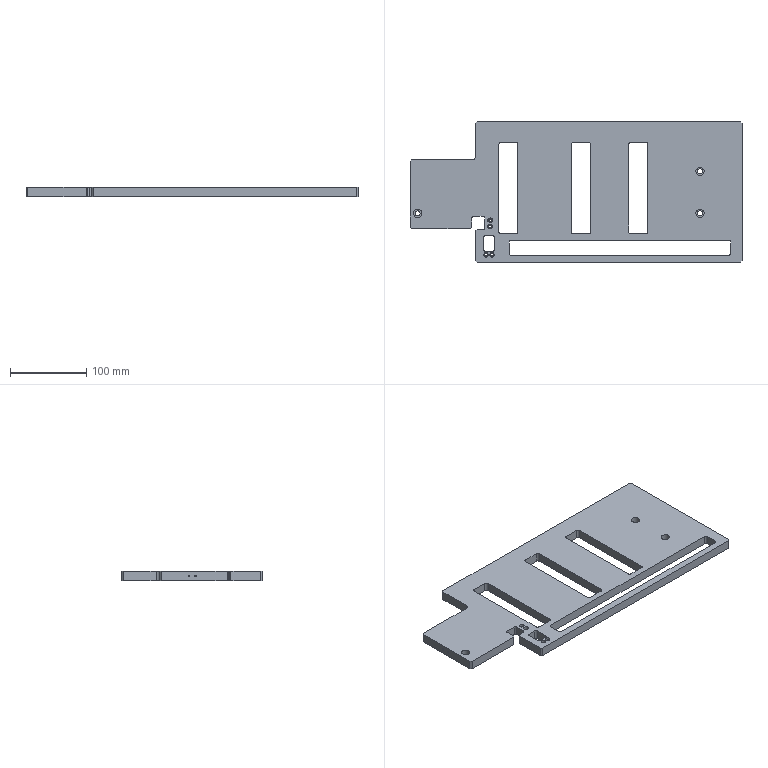NC program | NX | posted with a generic post | part box 435 x 184 x 12 mm
Lines 1 to 1792 of 10210:
N10 G17 G21 G94 G90
(DRILLING_COPY_1 , TOOL : D6A45)
N12 T01 M6
N14 G54
N16 G17 G0 G90 X-207.5 Y-28. S5000 M3
N18 G43 Z30. H1
N20 G94 G81 G98 Z-1. F350. R3.
N22 X-112.5 Y-37.
N24 Y-45.
N26 X-118. Y-82.5
N28 X-110.
N30 X162.5 Y-28.
N32 Y27.
N34 G80
N36 G0 X162.5 Y27. Z30.
N38 M5
(DRILLING_COPY_1_COPY_COPY_1 , TOOL : 3.5ZT)
N40 T07 M6
N42 G54
N44 G17 G0 G90 X-112.5 Y-37. S2000 M3
N46 G43 Z30. H7
N48 G94 G83 G98 Z-14.052 F200. Q2. R3.
N50 Y-45.
N52 X-110. Y-82.5
N54 X-118.
N56 G80
N58 G0 X-118. Y-82.5 Z30.
N60 M5
(DRILLING_COPY_1_COPY_COPY_1_COPY , TOOL : 6.5ZT)
N62 T16 M6
N64 G54
N66 G17 G0 G90 X-207.5 Y-28. S2000 M3
N68 G43 Z30. H16
N70 G94 G83 G98 Z-14.953 F200. Q2. R3.
N72 X162.5
N74 Y27.
N76 G80
N78 G0 X162.5 Y27. Z30.
N80 M5
(ZLEVEL_PROFILE_COPY_1_COPY_COPY_1_COPY , TOOL : D10)
N82 T15 M6
N84 G54
N86 G17 G0 G90 X-132.526 Y98.746 S9500 M3
N88 G43 Z30. H15
N90 Z0.
N92 G94 G1 Z-1. F1000.
N94 X-132.136 Y97.282
N96 G2 X-132.396 Y96.317 R1.
N98 G3 X-132.523 Y96.108 R0.16 F2000.
N100 X-133.106 Y95.606 R5.1
N102 G1 X-135.106 Y93.606
N104 G3 X-136.6 Y90. R5.1
N106 G1 Y47.203
N108 X-136.611 Y47.1
N110 X-215.5
N112 G3 X-219.106 Y45.606 R5.1
N114 G1 X-220.39 Y44.318
N116 X-220.664 Y44.045
N118 X-220.688 Y43.981
N120 G3 X-222.6 Y40. R5.1
N122 G1 Y-44.953
N124 X-222.597 Y-45.002
N126 Y-45.389
N128 X-222.569 Y-45.44
N130 G3 X-221.106 Y-49.606 R5.1
N132 G1 X-219.106 Y-51.606
N134 G3 X-215.5 Y-53.1 R5.1
N136 G1 X-138.5
N138 G3 X-136.6 Y-52.733 R5.1
N140 G1 Y-90.
N142 G3 X-135.106 Y-93.606 R5.1
N144 G1 X-133.106 Y-95.606
N146 G3 X-132.695 Y-95.975 R5.1
N148 G2 X-132.514 Y-96.441 R0.5
N150 G1 X-132.838 Y-98.537
N152 Z0.
N154 G0 Z54.
N156 X-132.526 Y98.746
N158 Z-1.
N160 G1 Z-2. F1000.
N162 X-132.136 Y97.282
N164 G2 X-132.396 Y96.317 R1.
N166 G3 X-132.523 Y96.108 R0.16 F2000.
N168 X-133.106 Y95.606 R5.1
N170 G1 X-135.106 Y93.606
N172 G3 X-136.6 Y90. R5.1
N174 G1 Y47.203
N176 X-136.611 Y47.1
N178 X-215.5
N180 G3 X-219.106 Y45.606 R5.1
N182 G1 X-220.39 Y44.318
N184 X-220.664 Y44.045
N186 X-220.688 Y43.981
N188 G3 X-222.6 Y40. R5.1
N190 G1 Y-44.953
N192 X-222.597 Y-45.002
N194 Y-45.389
N196 X-222.569 Y-45.44
N198 G3 X-221.106 Y-49.606 R5.1
N200 G1 X-219.106 Y-51.606
N202 G3 X-215.5 Y-53.1 R5.1
N204 G1 X-138.5
N206 G3 X-136.6 Y-52.733 R5.1
N208 G1 Y-90.
N210 G3 X-135.106 Y-93.606 R5.1
N212 G1 X-133.106 Y-95.606
N214 G3 X-132.695 Y-95.975 R5.1
N216 G2 X-132.514 Y-96.441 R0.5
N218 G1 X-132.838 Y-98.537
N220 Z-1.
N222 G0 Z54.
N224 X-132.526 Y98.746
N226 Z-2.
N228 G1 Z-3. F1000.
N230 X-132.136 Y97.282
N232 G2 X-132.396 Y96.317 R1.
N234 G3 X-132.523 Y96.108 R0.16 F2000.
N236 X-133.106 Y95.606 R5.1
N238 G1 X-135.106 Y93.606
N240 G3 X-136.6 Y90. R5.1
N242 G1 Y47.203
N244 X-136.611 Y47.1
N246 X-215.5
N248 G3 X-219.106 Y45.606 R5.1
N250 G1 X-220.39 Y44.318
N252 X-220.664 Y44.045
N254 X-220.688 Y43.981
N256 G3 X-222.6 Y40. R5.1
N258 G1 Y-44.953
N260 X-222.597 Y-45.002
N262 Y-45.389
N264 X-222.569 Y-45.44
N266 G3 X-221.106 Y-49.606 R5.1
N268 G1 X-219.106 Y-51.606
N270 G3 X-215.5 Y-53.1 R5.1
N272 G1 X-138.5
N274 G3 X-136.6 Y-52.733 R5.1
N276 G1 Y-90.
N278 G3 X-135.106 Y-93.606 R5.1
N280 G1 X-133.106 Y-95.606
N282 G3 X-132.695 Y-95.975 R5.1
N284 G2 X-132.514 Y-96.441 R0.5
N286 G1 X-132.838 Y-98.537
N288 Z-2.
N290 G0 Z54.
N292 X-132.526 Y98.746
N294 Z-3.
N296 G1 Z-4. F1000.
N298 X-132.136 Y97.282
N300 G2 X-132.396 Y96.317 R1.
N302 G3 X-132.523 Y96.108 R0.16 F2000.
N304 X-133.106 Y95.606 R5.1
N306 G1 X-135.106 Y93.606
N308 G3 X-136.6 Y90. R5.1
N310 G1 Y47.203
N312 X-136.611 Y47.1
N314 X-215.5
N316 G3 X-219.106 Y45.606 R5.1
N318 G1 X-220.39 Y44.318
N320 X-220.664 Y44.045
N322 X-220.688 Y43.981
N324 G3 X-222.6 Y40. R5.1
N326 G1 Y-44.953
N328 X-222.597 Y-45.002
N330 Y-45.389
N332 X-222.569 Y-45.44
N334 G3 X-221.106 Y-49.606 R5.1
N336 G1 X-219.106 Y-51.606
N338 G3 X-215.5 Y-53.1 R5.1
N340 G1 X-138.5
N342 G3 X-136.6 Y-52.733 R5.1
N344 G1 Y-90.
N346 G3 X-135.106 Y-93.606 R5.1
N348 G1 X-133.106 Y-95.606
N350 G3 X-132.695 Y-95.975 R5.1
N352 G2 X-132.514 Y-96.441 R0.5
N354 G1 X-132.838 Y-98.537
N356 Z-3.
N358 G0 Z54.
N360 X-132.526 Y98.746
N362 Z-4.
N364 G1 Z-5. F1000.
N366 X-132.136 Y97.282
N368 G2 X-132.396 Y96.317 R1.
N370 G3 X-132.523 Y96.108 R0.16 F2000.
N372 X-133.106 Y95.606 R5.1
N374 G1 X-135.106 Y93.606
N376 G3 X-136.6 Y90. R5.1
N378 G1 Y47.203
N380 X-136.611 Y47.1
N382 X-215.5
N384 G3 X-219.106 Y45.606 R5.1
N386 G1 X-220.39 Y44.318
N388 X-220.664 Y44.045
N390 X-220.688 Y43.981
N392 G3 X-222.6 Y40. R5.1
N394 G1 Y-44.953
N396 X-222.597 Y-45.002
N398 Y-45.389
N400 X-222.569 Y-45.44
N402 G3 X-221.106 Y-49.606 R5.1
N404 G1 X-219.106 Y-51.606
N406 G3 X-215.5 Y-53.1 R5.1
N408 G1 X-138.5
N410 G3 X-136.6 Y-52.733 R5.1
N412 G1 Y-90.
N414 G3 X-135.106 Y-93.606 R5.1
N416 G1 X-133.106 Y-95.606
N418 G3 X-132.695 Y-95.975 R5.1
N420 G2 X-132.514 Y-96.441 R0.5
N422 G1 X-132.838 Y-98.537
N424 Z-4.
N426 G0 Z54.
N428 X-132.526 Y98.746
N430 Z-5.
N432 G1 Z-6. F1000.
N434 X-132.136 Y97.282
N436 G2 X-132.396 Y96.317 R1.
N438 G3 X-132.523 Y96.108 R0.16 F2000.
N440 X-133.106 Y95.606 R5.1
N442 G1 X-135.106 Y93.606
N444 G3 X-136.6 Y90. R5.1
N446 G1 Y47.203
N448 X-136.611 Y47.1
N450 X-215.5
N452 G3 X-219.106 Y45.606 R5.1
N454 G1 X-220.39 Y44.318
N456 X-220.664 Y44.045
N458 X-220.688 Y43.981
N460 G3 X-222.6 Y40. R5.1
N462 G1 Y-44.953
N464 X-222.597 Y-45.002
N466 Y-45.389
N468 X-222.569 Y-45.44
N470 G3 X-221.106 Y-49.606 R5.1
N472 G1 X-219.106 Y-51.606
N474 G3 X-215.5 Y-53.1 R5.1
N476 G1 X-138.5
N478 G3 X-136.6 Y-52.733 R5.1
N480 G1 Y-90.
N482 G3 X-135.106 Y-93.606 R5.1
N484 G1 X-133.106 Y-95.606
N486 G3 X-132.695 Y-95.975 R5.1
N488 G2 X-132.514 Y-96.441 R0.5
N490 G1 X-132.838 Y-98.537
N492 Z-5.
N494 G0 Z54.
N496 X-132.526 Y98.746
N498 Z-6.
N500 G1 Z-7. F1000.
N502 X-132.136 Y97.282
N504 G2 X-132.396 Y96.317 R1.
N506 G3 X-132.523 Y96.108 R0.16 F2000.
N508 X-133.106 Y95.606 R5.1
N510 G1 X-135.106 Y93.606
N512 G3 X-136.6 Y90. R5.1
N514 G1 Y47.203
N516 X-136.611 Y47.1
N518 X-215.5
N520 G3 X-219.106 Y45.606 R5.1
N522 G1 X-220.39 Y44.318
N524 X-220.664 Y44.045
N526 X-220.688 Y43.981
N528 G3 X-222.6 Y40. R5.1
N530 G1 Y-44.953
N532 X-222.597 Y-45.002
N534 Y-45.389
N536 X-222.569 Y-45.44
N538 G3 X-221.106 Y-49.606 R5.1
N540 G1 X-219.106 Y-51.606
N542 G3 X-215.5 Y-53.1 R5.1
N544 G1 X-138.5
N546 G3 X-136.6 Y-52.733 R5.1
N548 G1 Y-90.
N550 G3 X-135.106 Y-93.606 R5.1
N552 G1 X-133.106 Y-95.606
N554 G3 X-132.695 Y-95.975 R5.1
N556 G2 X-132.514 Y-96.441 R0.5
N558 G1 X-132.838 Y-98.537
N560 Z-6.
N562 G0 Z54.
N564 X-132.526 Y98.746
N566 Z-7.
N568 G1 Z-8. F1000.
N570 X-132.136 Y97.282
N572 G2 X-132.396 Y96.317 R1.
N574 G3 X-132.523 Y96.108 R0.16 F2000.
N576 X-133.106 Y95.606 R5.1
N578 G1 X-135.106 Y93.606
N580 G3 X-136.6 Y90. R5.1
N582 G1 Y47.203
N584 X-136.611 Y47.1
N586 X-215.5
N588 G3 X-219.106 Y45.606 R5.1
N590 G1 X-220.39 Y44.318
N592 X-220.664 Y44.045
N594 X-220.688 Y43.981
N596 G3 X-222.6 Y40. R5.1
N598 G1 Y-44.953
N600 X-222.597 Y-45.002
N602 Y-45.389
N604 X-222.569 Y-45.44
N606 G3 X-221.106 Y-49.606 R5.1
N608 G1 X-219.106 Y-51.606
N610 G3 X-215.5 Y-53.1 R5.1
N612 G1 X-138.5
N614 G3 X-136.6 Y-52.733 R5.1
N616 G1 Y-90.
N618 G3 X-135.106 Y-93.606 R5.1
N620 G1 X-133.106 Y-95.606
N622 G3 X-132.695 Y-95.975 R5.1
N624 G2 X-132.514 Y-96.441 R0.5
N626 G1 X-132.838 Y-98.537
N628 Z-7.
N630 G0 Z54.
N632 X-132.526 Y98.746
N634 Z-8.
N636 G1 Z-9. F1000.
N638 X-132.136 Y97.282
N640 G2 X-132.396 Y96.317 R1.
N642 G3 X-132.523 Y96.108 R0.16 F2000.
N644 X-133.106 Y95.606 R5.1
N646 G1 X-135.106 Y93.606
N648 G3 X-136.6 Y90. R5.1
N650 G1 Y47.203
N652 X-136.611 Y47.1
N654 X-215.5
N656 G3 X-219.106 Y45.606 R5.1
N658 G1 X-220.39 Y44.318
N660 X-220.664 Y44.045
N662 X-220.688 Y43.981
N664 G3 X-222.6 Y40. R5.1
N666 G1 Y-44.953
N668 X-222.597 Y-45.002
N670 Y-45.389
N672 X-222.569 Y-45.44
N674 G3 X-221.106 Y-49.606 R5.1
N676 G1 X-219.106 Y-51.606
N678 G3 X-215.5 Y-53.1 R5.1
N680 G1 X-138.5
N682 G3 X-136.6 Y-52.733 R5.1
N684 G1 Y-90.
N686 G3 X-135.106 Y-93.606 R5.1
N688 G1 X-133.106 Y-95.606
N690 G3 X-132.695 Y-95.975 R5.1
N692 G2 X-132.514 Y-96.441 R0.5
N694 G1 X-132.838 Y-98.537
N696 Z-8.
N698 G0 Z54.
N700 X-132.526 Y98.746
N702 Z-9.
N704 G1 Z-10. F1000.
N706 X-132.136 Y97.282
N708 G2 X-132.396 Y96.317 R1.
N710 G3 X-132.523 Y96.108 R0.16 F2000.
N712 X-133.106 Y95.606 R5.1
N714 G1 X-135.106 Y93.606
N716 G3 X-136.6 Y90. R5.1
N718 G1 Y47.203
N720 X-136.611 Y47.1
N722 X-215.5
N724 G3 X-219.106 Y45.606 R5.1
N726 G1 X-220.39 Y44.318
N728 X-220.664 Y44.045
N730 X-220.688 Y43.981
N732 G3 X-222.6 Y40. R5.1
N734 G1 Y-44.953
N736 X-222.597 Y-45.002
N738 Y-45.389
N740 X-222.569 Y-45.44
N742 G3 X-221.106 Y-49.606 R5.1
N744 G1 X-219.106 Y-51.606
N746 G3 X-215.5 Y-53.1 R5.1
N748 G1 X-138.5
N750 G3 X-136.6 Y-52.733 R5.1
N752 G1 Y-90.
N754 G3 X-135.106 Y-93.606 R5.1
N756 G1 X-133.106 Y-95.606
N758 G3 X-132.695 Y-95.975 R5.1
N760 G2 X-132.514 Y-96.441 R0.5
N762 G1 X-132.838 Y-98.537
N764 Z-9.
N766 G0 Z54.
N768 X-132.526 Y98.746
N770 Z-10.
N772 G1 Z-11. F1000.
N774 X-132.136 Y97.282
N776 G2 X-132.396 Y96.317 R1.
N778 G3 X-132.523 Y96.108 R0.16 F2000.
N780 X-133.106 Y95.606 R5.1
N782 G1 X-135.106 Y93.606
N784 G3 X-136.6 Y90. R5.1
N786 G1 Y47.203
N788 X-136.611 Y47.1
N790 X-215.5
N792 G3 X-219.106 Y45.606 R5.1
N794 G1 X-220.39 Y44.318
N796 X-220.664 Y44.045
N798 X-220.688 Y43.981
N800 G3 X-222.6 Y40. R5.1
N802 G1 Y-44.953
N804 X-222.597 Y-45.002
N806 Y-45.389
N808 X-222.569 Y-45.44
N810 G3 X-221.106 Y-49.606 R5.1
N812 G1 X-219.106 Y-51.606
N814 G3 X-215.5 Y-53.1 R5.1
N816 G1 X-138.5
N818 G3 X-136.6 Y-52.733 R5.1
N820 G1 Y-90.
N822 G3 X-135.106 Y-93.606 R5.1
N824 G1 X-133.106 Y-95.606
N826 G3 X-132.695 Y-95.975 R5.1
N828 G2 X-132.514 Y-96.441 R0.5
N830 G1 X-132.838 Y-98.537
N832 Z-10.
N834 G0 Z54.
N836 X-132.526 Y98.746
N838 Z-11.
N840 G1 Z-12. F1000.
N842 X-132.136 Y97.282
N844 G2 X-132.396 Y96.317 R1.
N846 G3 X-132.523 Y96.108 R0.16 F2000.
N848 X-133.106 Y95.606 R5.1
N850 G1 X-135.106 Y93.606
N852 G3 X-136.6 Y90. R5.1
N854 G1 Y47.203
N856 X-136.611 Y47.1
N858 X-215.5
N860 G3 X-219.106 Y45.606 R5.1
N862 G1 X-220.39 Y44.318
N864 X-220.664 Y44.045
N866 X-220.688 Y43.981
N868 G3 X-222.6 Y40. R5.1
N870 G1 Y-44.953
N872 X-222.597 Y-45.002
N874 Y-45.389
N876 X-222.569 Y-45.44
N878 G3 X-221.106 Y-49.606 R5.1
N880 G1 X-219.106 Y-51.606
N882 G3 X-215.5 Y-53.1 R5.1
N884 G1 X-138.5
N886 G3 X-136.6 Y-52.733 R5.1
N888 G1 Y-90.
N890 G3 X-135.106 Y-93.606 R5.1
N892 G1 X-133.106 Y-95.606
N894 G3 X-132.695 Y-95.975 R5.1
N896 G2 X-132.514 Y-96.441 R0.5
N898 G1 X-132.838 Y-98.537
N900 Z-11.
N902 G0 Z30.
(ZLEVEL_PROFILE_COPY_1_COPY_COPY_1_COPY_COPY , TOOL : D10)
N904 X218.504 Y98.759
N906 Z0.
N908 G1 Z-1. F1000.
N910 X218.121 Y97.287
N912 G3 X218.386 Y96.323 R1.
N914 G1 X218.708 Y96.005 F3000.
N916 X218.733 Y95.985
N918 X218.71 Y95.963
N920 G2 X219.106 Y95.606 R5.1
N922 G1 X220.495 Y94.217
N924 X220.554 Y94.173
N926 X220.524 Y94.107
N928 G2 X222.6 Y90. R5.1
N930 G1 Y-90.
N932 G2 X221.106 Y-93.606 R5.1
N934 G1 X219.106 Y-95.606
N936 X218.386 Y-96.323
N938 G3 X218.125 Y-97.289 R1.
N940 G1 X218.514 Y-98.752
N942 Z0.
N944 G0 Z30.
N946 Z-1.
N948 G1 Z-2. F1000.
N950 X218.125 Y-97.289
N952 G2 X218.386 Y-96.323 R1.
N954 G1 X219.106 Y-95.606 F3000.
N956 X221.106 Y-93.606
N958 G3 X222.6 Y-90. R5.1
N960 G1 Y90.
N962 G3 X220.524 Y94.107 R5.1
N964 G1 X220.554 Y94.173
N966 X220.495 Y94.217
N968 X219.106 Y95.606
N970 G3 X218.71 Y95.963 R5.1
N972 G1 X218.733 Y95.985
N974 X218.708 Y96.005
N976 X218.386 Y96.323
N978 G2 X218.121 Y97.287 R1.
N980 G1 X218.504 Y98.759
N982 Z-1.
N984 G0 Z30.
N986 Z-2.
N988 G1 Z-3. F1000.
N990 X218.121 Y97.287
N992 G3 X218.386 Y96.323 R1.
N994 G1 X218.708 Y96.005 F3000.
N996 X218.733 Y95.985
N998 X218.71 Y95.963
N1000 G2 X219.106 Y95.606 R5.1
N1002 G1 X220.495 Y94.217
N1004 X220.554 Y94.173
N1006 X220.524 Y94.107
N1008 G2 X222.6 Y90. R5.1
N1010 G1 Y-90.
N1012 G2 X221.106 Y-93.606 R5.1
N1014 G1 X219.106 Y-95.606
N1016 X218.386 Y-96.323
N1018 G3 X218.125 Y-97.289 R1.
N1020 G1 X218.514 Y-98.752
N1022 Z-2.
N1024 G0 Z30.
N1026 Z-3.
N1028 G1 Z-4. F1000.
N1030 X218.125 Y-97.289
N1032 G2 X218.386 Y-96.323 R1.
N1034 G1 X219.106 Y-95.606 F3000.
N1036 X221.106 Y-93.606
N1038 G3 X222.6 Y-90. R5.1
N1040 G1 Y90.
N1042 G3 X220.524 Y94.107 R5.1
N1044 G1 X220.554 Y94.173
N1046 X220.495 Y94.217
N1048 X219.106 Y95.606
N1050 G3 X218.71 Y95.963 R5.1
N1052 G1 X218.733 Y95.985
N1054 X218.708 Y96.005
N1056 X218.386 Y96.323
N1058 G2 X218.121 Y97.287 R1.
N1060 G1 X218.504 Y98.759
N1062 Z-3.
N1064 G0 Z30.
N1066 Z-4.
N1068 G1 Z-5. F1000.
N1070 X218.121 Y97.287
N1072 G3 X218.386 Y96.323 R1.
N1074 G1 X218.708 Y96.005 F3000.
N1076 X218.733 Y95.985
N1078 X218.71 Y95.963
N1080 G2 X219.106 Y95.606 R5.1
N1082 G1 X220.495 Y94.217
N1084 X220.554 Y94.173
N1086 X220.524 Y94.107
N1088 G2 X222.6 Y90. R5.1
N1090 G1 Y-90.
N1092 G2 X221.106 Y-93.606 R5.1
N1094 G1 X219.106 Y-95.606
N1096 X218.386 Y-96.323
N1098 G3 X218.125 Y-97.289 R1.
N1100 G1 X218.514 Y-98.752
N1102 Z-4.
N1104 G0 Z30.
N1106 Z-5.
N1108 G1 Z-6. F1000.
N1110 X218.125 Y-97.289
N1112 G2 X218.386 Y-96.323 R1.
N1114 G1 X219.106 Y-95.606 F3000.
N1116 X221.106 Y-93.606
N1118 G3 X222.6 Y-90. R5.1
N1120 G1 Y90.
N1122 G3 X220.524 Y94.107 R5.1
N1124 G1 X220.554 Y94.173
N1126 X220.495 Y94.217
N1128 X219.106 Y95.606
N1130 G3 X218.71 Y95.963 R5.1
N1132 G1 X218.733 Y95.985
N1134 X218.708 Y96.005
N1136 X218.386 Y96.323
N1138 G2 X218.121 Y97.287 R1.
N1140 G1 X218.504 Y98.759
N1142 Z-5.
N1144 G0 Z30.
N1146 Z-6.
N1148 G1 Z-7. F1000.
N1150 X218.121 Y97.287
N1152 G3 X218.386 Y96.323 R1.
N1154 G1 X218.708 Y96.005 F3000.
N1156 X218.733 Y95.985
N1158 X218.71 Y95.963
N1160 G2 X219.106 Y95.606 R5.1
N1162 G1 X220.495 Y94.217
N1164 X220.554 Y94.173
N1166 X220.524 Y94.107
N1168 G2 X222.6 Y90. R5.1
N1170 G1 Y-90.
N1172 G2 X221.106 Y-93.606 R5.1
N1174 G1 X219.106 Y-95.606
N1176 X218.386 Y-96.323
N1178 G3 X218.125 Y-97.289 R1.
N1180 G1 X218.514 Y-98.752
N1182 Z-6.
N1184 G0 Z30.
N1186 Z-7.
N1188 G1 Z-8. F1000.
N1190 X218.126 Y-97.289
N1192 G2 X218.386 Y-96.323 R1.
N1194 G1 X219.106 Y-95.606 F3000.
N1196 X221.106 Y-93.606
N1198 G3 X222.6 Y-90. R5.1
N1200 G1 Y90.
N1202 G3 X220.524 Y94.107 R5.1
N1204 G1 X220.554 Y94.173
N1206 X220.495 Y94.217
N1208 X219.106 Y95.606
N1210 G3 X218.71 Y95.963 R5.1
N1212 G1 X218.733 Y95.985
N1214 X218.708 Y96.005
N1216 X218.386 Y96.323
N1218 G2 X218.121 Y97.287 R1.
N1220 G1 X218.504 Y98.759
N1222 Z-7.
N1224 G0 Z30.
N1226 Z-8.
N1228 G1 Z-9. F1000.
N1230 X218.121 Y97.287
N1232 G3 X218.386 Y96.323 R1.
N1234 G1 X218.708 Y96.005 F3000.
N1236 X218.733 Y95.985
N1238 X218.71 Y95.963
N1240 G2 X219.106 Y95.606 R5.1
N1242 G1 X220.495 Y94.217
N1244 X220.554 Y94.173
N1246 X220.524 Y94.107
N1248 G2 X222.6 Y90. R5.1
N1250 G1 Y-90.
N1252 G2 X221.106 Y-93.606 R5.1
N1254 G1 X219.106 Y-95.606
N1256 X218.386 Y-96.323
N1258 G3 X218.126 Y-97.289 R1.
N1260 G1 X218.514 Y-98.752
N1262 Z-8.
N1264 G0 Z30.
N1266 Z-9.
N1268 G1 Z-10. F1000.
N1270 X218.126 Y-97.289
N1272 G2 X218.386 Y-96.323 R1.
N1274 G1 X219.106 Y-95.606 F3000.
N1276 X221.106 Y-93.606
N1278 G3 X222.6 Y-90. R5.1
N1280 G1 Y90.
N1282 G3 X220.524 Y94.107 R5.1
N1284 G1 X220.554 Y94.173
N1286 X220.495 Y94.217
N1288 X219.106 Y95.606
N1290 G3 X218.71 Y95.963 R5.1
N1292 G1 X218.733 Y95.985
N1294 X218.708 Y96.005
N1296 X218.386 Y96.323
N1298 G2 X218.121 Y97.287 R1.
N1300 G1 X218.504 Y98.759
N1302 Z-9.
N1304 G0 Z30.
N1306 Z-10.
N1308 G1 Z-11. F1000.
N1310 X218.121 Y97.287
N1312 G3 X218.386 Y96.323 R1.
N1314 G1 X218.708 Y96.005 F3000.
N1316 X218.733 Y95.985
N1318 X218.71 Y95.963
N1320 G2 X219.106 Y95.606 R5.1
N1322 G1 X220.495 Y94.217
N1324 X220.554 Y94.173
N1326 X220.524 Y94.107
N1328 G2 X222.6 Y90. R5.1
N1330 G1 Y-90.
N1332 G2 X221.106 Y-93.606 R5.1
N1334 G1 X219.106 Y-95.606
N1336 X218.386 Y-96.323
N1338 G3 X218.126 Y-97.289 R1.
N1340 G1 X218.514 Y-98.752
N1342 Z-10.
N1344 G0 Z30.
N1346 Z-11.
N1348 G1 Z-12. F1000.
N1350 X218.126 Y-97.289
N1352 G2 X218.386 Y-96.323 R1.
N1354 G1 X219.106 Y-95.606 F3000.
N1356 X221.106 Y-93.606
N1358 G3 X222.6 Y-90. R5.1
N1360 G1 Y90.
N1362 G3 X220.524 Y94.107 R5.1
N1364 G1 X220.554 Y94.173
N1366 X220.495 Y94.217
N1368 X219.106 Y95.606
N1370 G3 X218.71 Y95.963 R5.1
N1372 G1 X218.733 Y95.985
N1374 X218.708 Y96.005
N1376 X218.386 Y96.323
N1378 G2 X218.121 Y97.287 R1.
N1380 G1 X218.504 Y98.759
N1382 Z-11.
N1384 G0 Z30.
(ZLEVEL_PROFILE_COPY_1_COPY_COPY_1_COPY_COPY_COPY , TOOL : D10)
N1386 X-44.497 Y-68.1
N1388 Z1.5
N1390 G1 X-82.4 Z-0.486 F1000.
N1392 Y-77.9 Z-1.
N1394 X197.4 F3000.
N1396 Y-68.1
N1398 X-82.4
N1400 Y-77.9
N1402 X-25.11 Z-2.
N1404 X197.4
N1406 Y-68.1
N1408 X-82.4
N1410 Y-77.9
N1412 X-25.11 Z-3.
N1414 X197.4
N1416 Y-68.1
N1418 X-82.4
N1420 Y-77.9
N1422 X-25.11 Z-4.
N1424 X197.4
N1426 Y-68.1
N1428 X-82.4
N1430 Y-77.9
N1432 X-25.11 Z-5.
N1434 X197.4
N1436 Y-68.1
N1438 X-82.4
N1440 Y-77.9
N1442 X-25.11 Z-6.
N1444 X197.4
N1446 Y-68.1
N1448 X-82.4
N1450 Y-77.9
N1452 X-25.11 Z-7.
N1454 X197.4
N1456 Y-68.1
N1458 X-82.4
N1460 Y-77.9
N1462 X-25.11 Z-8.
N1464 X197.4
N1466 Y-68.1
N1468 X-82.4
N1470 Y-77.9
N1472 X-25.11 Z-9.
N1474 X197.4
N1476 Y-68.1
N1478 X-82.4
N1480 Y-77.9
N1482 X-25.11 Z-10.
N1484 X197.4
N1486 Y-68.1
N1488 X-82.4
N1490 Y-77.9
N1492 X-25.11 Z-11.
N1494 X197.4
N1496 Y-68.1
N1498 X-82.4
N1500 Y-77.9
N1502 X-25.11 Z-12.
N1504 X197.4
N1506 Y-68.1
N1508 X-82.4
N1510 Y-77.9
N1512 X-25.11
N1514 Z-10.5
N1516 G0 Z30.
(ZLEVEL_PROFILE_COPY_1_COPY_COPY_1_COPY_COPY_COPY_COPY , TOOL : D10)
N1518 X-115.503 Y-72.4
N1520 Z1.5
N1522 G1 X-111.6 Z1.295 F1000.
N1524 Y-62.6 Z0.782
N1526 X-116.4 Z0.53
N1528 Y-72.4 Z0.017
N1530 X-111.6 Z-0.235
N1532 Y-62.6 Z-0.748
N1534 X-116.4 Z-1.
N1536 Y-72.4 F3000.
N1538 X-111.6
N1540 Y-62.6
N1542 X-116.4
N1544 Y-72.205 Z-1.439
N1546 X-116.211 Y-72.4 Z-1.456
N1548 X-111.6 Z-1.667
N1550 Y-65.1 Z-2.
N1552 Y-62.6
N1554 X-116.4
N1556 Y-72.205 Z-2.439
N1558 X-116.211 Y-72.4 Z-2.456
N1560 X-111.6 Z-2.667
N1562 Y-65.1 Z-3.
N1564 Y-62.6
N1566 X-116.4
N1568 Y-72.205 Z-3.439
N1570 X-116.211 Y-72.4 Z-3.456
N1572 X-111.6 Z-3.667
N1574 Y-65.1 Z-4.
N1576 Y-62.6
N1578 X-116.4
N1580 Y-72.205 Z-4.439
N1582 X-116.211 Y-72.4 Z-4.456
N1584 X-111.6 Z-4.667
N1586 Y-65.1 Z-5.
N1588 Y-62.6
N1590 X-116.4
N1592 Y-72.205 Z-5.439
N1594 X-116.211 Y-72.4 Z-5.456
N1596 X-111.6 Z-5.667
N1598 Y-65.1 Z-6.
N1600 Y-62.6
N1602 X-116.4
N1604 Y-72.205 Z-6.439
N1606 X-116.211 Y-72.4 Z-6.456
N1608 X-111.6 Z-6.667
N1610 Y-65.1 Z-7.
N1612 Y-62.6
N1614 X-116.4
N1616 Y-72.205 Z-7.439
N1618 X-116.211 Y-72.4 Z-7.456
N1620 X-111.6 Z-7.667
N1622 Y-65.1 Z-8.
N1624 Y-62.6
N1626 X-116.4
N1628 Y-72.205 Z-8.439
N1630 X-116.211 Y-72.4 Z-8.456
N1632 X-111.6 Z-8.667
N1634 Y-65.1 Z-9.
N1636 Y-62.6
N1638 X-116.4
N1640 Y-72.205 Z-9.439
N1642 X-116.211 Y-72.4 Z-9.456
N1644 X-111.6 Z-9.667
N1646 Y-65.1 Z-10.
N1648 Y-62.6
N1650 X-116.4
N1652 Y-72.205 Z-10.439
N1654 X-116.211 Y-72.4 Z-10.456
N1656 X-111.6 Z-10.667
N1658 Y-65.1 Z-11.
N1660 Y-62.6
N1662 X-116.4
N1664 Y-72.205 Z-11.439
N1666 X-116.211 Y-72.4 Z-11.456
N1668 X-111.6 Z-11.667
N1670 Y-65.1 Z-12.
N1672 Y-62.6
N1674 X-116.4
N1676 Y-72.4
N1678 X-111.6
N1680 Y-65.1
N1682 Z-10.5
N1684 G0 Z30.
(ZLEVEL_PROFILE_COPY_1_COPY_COPY_1_COPY_COPY_COPY_COPY_COPY , TOOL : D10)
N1686 X-124.6 Y-41.326
N1688 Z1.5
N1690 G1 Y-37.1 Z1.279 F1000.
N1692 X-131.4 Z0.922
N1694 Y-40.976 Z0.719
N1696 X-131.401 Y-43.961 Z0.563
N1698 X-131.343 Z0.559
N1700 X-130.321 Y-43.901 Z0.506
N1702 X-130.079 Z0.493
N1704 X-128.922 Y-43.933 Z0.433
N1706 X-128.87 Y-43.901 Z0.429
N1708 X-126.162 Y-43.9 Z0.287
N1710 X-124.6 Z0.206
N1712 Y-37.1 Z-0.151
N1714 X-131.4 Z-0.507
N1716 Y-40.976 Z-0.71
N1718 X-131.401 Y-43.961 Z-0.867
N1720 X-131.343 Z-0.87
N1722 X-130.321 Y-43.901 Z-0.923
N1724 X-130.079 Z-0.936
N1726 X-128.922 Y-43.933 Z-0.997
N1728 X-128.87 Y-43.901 Z-1.
N1730 X-126.162 Y-43.9 F3000.
N1732 X-124.6
N1734 Y-37.1
N1736 X-131.4
N1738 Y-40.976
N1740 X-131.401 Y-43.961
N1742 X-131.343
N1744 X-130.321 Y-43.901
N1746 X-130.079
N1748 X-128.922 Y-43.933
N1750 X-128.87 Y-43.901
N1752 X-128.492 Y-43.9 Z-1.019
N1754 X-128.113 Z-1.037
N1756 X-126.219 Z-1.13
N1758 X-125.84 Z-1.148
N1760 X-124.6 Z-1.209
N1762 Y-37.1 Z-1.541
N1764 X-131.4 Z-1.874
N1766 Y-39.685 Z-2.
N1768 Y-40.976
N1770 X-131.401 Y-43.961
N1772 X-131.343
N1774 X-130.321 Y-43.901
N1776 X-130.079
N1778 X-128.922 Y-43.933
N1780 X-128.871 Y-43.901
N1782 X-128.492 Y-43.9 Z-2.019
N1784 X-128.113 Z-2.037
N1786 X-126.219 Z-2.13
N1788 X-125.84 Z-2.148
N1790 X-124.6 Z-2.209
N1792 Y-37.1 Z-2.541
N1794 X-131.4 Z-2.874
N1796 Y-39.685 Z-3.
N1798 Y-40.976
N1800 X-131.401 Y-43.961
N1802 X-131.343
N1804 X-130.321 Y-43.901
N1806 X-130.079
N1808 X-128.922 Y-43.933
N1810 X-128.871 Y-43.901
N1812 X-128.492 Y-43.9 Z-3.019
N1814 X-128.113 Z-3.037
N1816 X-126.219 Z-3.13
N1818 X-125.84 Z-3.148
N1820 X-124.6 Z-3.209
N1822 Y-37.1 Z-3.541
N1824 X-131.4 Z-3.874
N1826 Y-39.685 Z-4.
N1828 Y-40.976
N1830 Y-43.961
N1832 X-131.343
N1834 X-130.321 Y-43.9
N1836 X-130.079
N1838 X-128.922 Y-43.933
N1840 X-128.871 Y-43.901
N1842 X-128.492 Y-43.9 Z-4.019
N1844 X-128.113 Z-4.037
N1846 X-126.219 Z-4.13
N1848 X-125.84 Z-4.148
N1850 X-124.6 Z-4.209
N1852 Y-37.1 Z-4.541
N1854 X-131.4 Z-4.874
N1856 Y-39.684 Z-5.
N1858 Y-40.976
N1860 Y-43.961
N1862 X-131.343
N1864 X-130.321 Y-43.9
N1866 X-130.079
N1868 X-128.922 Y-43.933
N1870 X-128.871 Y-43.9
N1872 X-128.492 Z-5.019
N1874 X-128.113 Z-5.037
N1876 X-126.219 Z-5.13
N1878 X-125.84 Z-5.148
N1880 X-124.6 Z-5.209
N1882 Y-37.1 Z-5.541
N1884 X-131.4 Z-5.874
N1886 Y-39.684 Z-6.
N1888 Y-40.976
N1890 Y-43.961
N1892 X-131.343
N1894 X-130.321 Y-43.9
N1896 X-130.079
N1898 X-128.922 Y-43.933
N1900 X-128.871 Y-43.9
N1902 X-128.492 Z-6.019
N1904 X-128.113 Z-6.037
N1906 X-126.219 Z-6.13
N1908 X-125.84 Z-6.148
N1910 X-124.6 Z-6.209
N1912 Y-37.1 Z-6.541
N1914 X-131.4 Z-6.874
N1916 Y-39.684 Z-7.
N1918 Y-40.976
N1920 Y-43.961
N1922 X-131.343
N1924 X-130.321 Y-43.9
N1926 X-130.079
N1928 X-128.922 Y-43.933
N1930 X-128.871 Y-43.9
N1932 X-128.492 Z-7.019
N1934 X-128.113 Z-7.037
N1936 X-126.219 Z-7.13
N1938 X-125.84 Z-7.148
N1940 X-124.6 Z-7.209
N1942 Y-37.1 Z-7.541
N1944 X-131.4 Z-7.874
N1946 Y-39.684 Z-8.
N1948 Y-40.976
N1950 Y-43.961
N1952 X-131.344
N1954 X-130.321 Y-43.9
N1956 X-130.079
N1958 X-128.922 Y-43.933
N1960 X-128.871 Y-43.9
N1962 X-128.492 Z-8.019
N1964 X-128.113 Z-8.037
N1966 X-126.219 Z-8.13
N1968 X-125.84 Z-8.148
N1970 X-124.6 Z-8.209
N1972 Y-37.1 Z-8.541
N1974 X-131.4 Z-8.874
N1976 Y-39.684 Z-9.
N1978 Y-40.976
N1980 Y-43.961
N1982 X-131.344
N1984 X-130.321 Y-43.9
N1986 X-130.079
N1988 X-128.922 Y-43.933
N1990 X-128.871 Y-43.9
N1992 X-128.492 Z-9.019
N1994 X-128.113 Z-9.037
N1996 X-126.219 Z-9.13
N1998 X-125.84 Z-9.148
N2000 X-124.6 Z-9.209
N2002 Y-37.1 Z-9.541
N2004 X-131.4 Z-9.874
N2006 Y-39.684 Z-10.
N2008 Y-40.976
N2010 Y-43.961
N2012 X-131.344
N2014 X-130.321 Y-43.9
N2016 X-130.079
N2018 X-128.922 Y-43.933
N2020 X-128.871 Y-43.9
N2022 X-128.492 Z-10.019
N2024 X-128.113 Z-10.037
N2026 X-126.219 Z-10.13
N2028 X-125.84 Z-10.148
N2030 X-124.6 Z-10.209
N2032 Y-37.1 Z-10.541
N2034 X-131.4 Z-10.874
N2036 Y-39.684 Z-11.
N2038 Y-40.976
N2040 Y-43.961
N2042 X-131.344
N2044 X-130.321 Y-43.9
N2046 X-130.079
N2048 X-128.922 Y-43.933
N2050 X-128.871 Y-43.9
N2052 X-128.492 Z-11.019
N2054 X-128.113 Z-11.037
N2056 X-126.219 Z-11.13
N2058 X-125.84 Z-11.148
N2060 X-124.6 Z-11.209
N2062 Y-37.1 Z-11.541
N2064 X-131.4 Z-11.874
N2066 Y-39.684 Z-12.
N2068 Y-40.976
N2070 Y-43.961
N2072 X-131.344
N2074 X-130.321 Y-43.9
N2076 X-130.079
N2078 X-128.922 Y-43.933
N2080 X-128.87 Y-43.9
N2082 X-126.162
N2084 X-124.6
N2086 Y-37.1
N2088 X-131.4
N2090 Y-39.684
N2092 Z-10.5
N2094 G0 Z30.
(CAVITY_MILL , TOOL : D10)
N2096 X80.1 Y49.841
N2098 Z1.5
N2100 G1 Y5. Z-0.85 F1000.
N2102 Y-43.9 F2500.
N2104 X82.9
N2106 Y53.9
N2108 X80.1
N2110 Y5.
N2112 X74.1
N2114 Y-49.9
N2116 X88.9
N2118 Y59.9
N2120 X74.1
N2122 Y5.
N2124 Z0.65
N2126 G0 X82.9 Y-39.841
N2128 G1 Y5. Z-1.7 F1000.
N2130 Y53.9 F2500.
N2132 X80.1
N2134 Y-43.9
N2136 X82.9
N2138 Y5.
N2140 X88.9
N2142 Y59.9
N2144 X74.1
N2146 Y-49.9
N2148 X88.9
N2150 Y5.
N2152 Z-0.2
N2154 G0 X82.9 Y-39.841
N2156 G1 Y5. Z-2.55 F1000.
N2158 Y53.9 F2500.
N2160 X80.1
N2162 Y-43.9
N2164 X82.9
N2166 Y5.
N2168 X88.9
N2170 Y59.9
N2172 X74.1
N2174 Y-49.9
N2176 X88.9
N2178 Y5.
N2180 Z-1.05
N2182 G0 X82.9 Y-39.841
N2184 G1 Y5. Z-3.4 F1000.
N2186 Y53.9 F2500.
N2188 X80.1
N2190 Y-43.9
N2192 X82.9
N2194 Y5.
N2196 X88.9
N2198 Y59.9
N2200 X74.1
N2202 Y-49.9
N2204 X88.9
N2206 Y5.
N2208 Z-1.9
N2210 G0 X82.9 Y-40.318
N2212 G1 Y5. Z-4.275 F1000.
N2214 Y53.9 F2500.
N2216 X80.1
N2218 Y-43.9
N2220 X82.9
N2222 Y5.
N2224 X88.9
N2226 Y59.9
N2228 X74.1
N2230 Y-49.9
N2232 X88.9
N2234 Y5.
N2236 Z-2.775
N2238 G0 X82.9 Y-40.318
N2240 G1 Y5. Z-5.15 F1000.
N2242 Y53.9 F2500.
N2244 X80.1
N2246 Y-43.9
N2248 X82.9
N2250 Y5.
N2252 X88.9
N2254 Y59.9
N2256 X74.1
N2258 Y-49.9
N2260 X88.9
N2262 Y5.
N2264 Z-3.65
N2266 G0 X82.9 Y-40.318
N2268 G1 Y5. Z-6.025 F1000.
N2270 Y53.9 F2500.
N2272 X80.1
N2274 Y-43.9
N2276 X82.9
N2278 Y5.
N2280 X88.9
N2282 Y59.9
N2284 X74.1
N2286 Y-49.9
N2288 X88.9
N2290 Y5.
N2292 Z-4.525
N2294 G0 X82.9 Y-40.318
N2296 G1 Y5. Z-6.9 F1000.
N2298 Y53.9 F2500.
N2300 X80.1
N2302 Y-43.9
N2304 X82.9
N2306 Y5.
N2308 X88.9
N2310 Y59.9
N2312 X74.1
N2314 Y-49.9
N2316 X88.9
N2318 Y5.
N2320 Z-5.4
N2322 G0 X82.9 Y-39.841
N2324 G1 Y5. Z-7.75 F1000.
N2326 Y53.9 F2500.
N2328 X80.1
N2330 Y-43.9
N2332 X82.9
N2334 Y5.
N2336 X88.9
N2338 Y59.9
N2340 X74.1
N2342 Y-49.9
N2344 X88.9
N2346 Y5.
N2348 Z-6.25
N2350 G0 X82.9 Y-39.841
N2352 G1 Y5. Z-8.6 F1000.
N2354 Y53.9 F2500.
N2356 X80.1
N2358 Y-43.9
N2360 X82.9
N2362 Y5.
N2364 X88.9
N2366 Y59.9
N2368 X74.1
N2370 Y-49.9
N2372 X88.9
N2374 Y5.
N2376 Z-7.1
N2378 G0 X82.9 Y-39.841
N2380 G1 Y5. Z-9.45 F1000.
N2382 Y53.9 F2500.
N2384 X80.1
N2386 Y-43.9
N2388 X82.9
N2390 Y5.
N2392 X88.9
N2394 Y59.9
N2396 X74.1
N2398 Y-49.9
N2400 X88.9
N2402 Y5.
N2404 Z-7.95
N2406 G0 X82.9 Y-39.841
N2408 G1 Y5. Z-10.3 F1000.
N2410 Y53.9 F2500.
N2412 X80.1
N2414 Y-43.9
N2416 X82.9
N2418 Y5.
N2420 X88.9
N2422 Y59.9
N2424 X74.1
N2426 Y-49.9
N2428 X88.9
N2430 Y5.
N2432 Z-8.8
N2434 G0 X82.9 Y-39.841
N2436 G1 Y5. Z-11.15 F1000.
N2438 Y53.9 F2500.
N2440 X80.1
N2442 Y-43.9
N2444 X82.9
N2446 Y5.
N2448 X88.9
N2450 Y59.9
N2452 X74.1
N2454 Y-49.9
N2456 X88.9
N2458 Y5.
N2460 Z-9.65
N2462 G0 X82.9 Y-39.841
N2464 G1 Y5. Z-12. F1000.
N2466 Y53.9 F2500.
N2468 X80.1
N2470 Y-43.9
N2472 X82.9
N2474 Y5.
N2476 X88.9
N2478 Y59.9
N2480 X74.1
N2482 Y-49.9
N2484 X88.9
N2486 Y5.
N2488 Z-10.5
N2490 G0 Z30.
N2492 X7.9 Y-39.841
N2494 Z1.5
N2496 G1 Y5. Z-0.85 F1000.
N2498 Y53.9 F2500.
N2500 X5.1
N2502 Y-43.9
N2504 X7.9
N2506 Y5.
N2508 X13.9
N2510 Y59.9
N2512 X-0.9
N2514 Y-49.9
N2516 X13.9
N2518 Y5.
N2520 Z0.65
N2522 G0 X7.9 Y-39.841
N2524 G1 Y5. Z-1.7 F1000.
N2526 Y53.9 F2500.
N2528 X5.1
N2530 Y-43.9
N2532 X7.9
N2534 Y5.
N2536 X13.9
N2538 Y59.9
N2540 X-0.9
N2542 Y-49.9
N2544 X13.9
N2546 Y5.
N2548 Z-0.2
N2550 G0 X7.9 Y-39.841
N2552 G1 Y5. Z-2.55 F1000.
N2554 Y53.9 F2500.
N2556 X5.1
N2558 Y-43.9
N2560 X7.9
N2562 Y5.
N2564 X13.9
N2566 Y59.9
N2568 X-0.9
N2570 Y-49.9
N2572 X13.9
N2574 Y5.
N2576 Z-1.05
N2578 G0 X7.9 Y-39.841
N2580 G1 Y5. Z-3.4 F1000.
N2582 Y53.9 F2500.
N2584 X5.1
N2586 Y-43.9
N2588 X7.9
N2590 Y5.
N2592 X13.9
N2594 Y59.9
N2596 X-0.9
N2598 Y-49.9
N2600 X13.9
N2602 Y5.
N2604 Z-1.9
N2606 G0 X7.9 Y-40.318
N2608 G1 Y5. Z-4.275 F1000.
N2610 Y53.9 F2500.
N2612 X5.1
N2614 Y-43.9
N2616 X7.9
N2618 Y5.
N2620 X13.9
N2622 Y59.9
N2624 X-0.9
N2626 Y-49.9
N2628 X13.9
N2630 Y5.
N2632 Z-2.775
N2634 G0 X7.9 Y-40.318
N2636 G1 Y5. Z-5.15 F1000.
N2638 Y53.9 F2500.
N2640 X5.1
N2642 Y-43.9
N2644 X7.9
N2646 Y5.
N2648 X13.9
N2650 Y59.9
N2652 X-0.9
N2654 Y-49.9
N2656 X13.9
N2658 Y5.
N2660 Z-3.65
N2662 G0 X7.9 Y-40.318
N2664 G1 Y5. Z-6.025 F1000.
N2666 Y53.9 F2500.
N2668 X5.1
N2670 Y-43.9
N2672 X7.9
N2674 Y5.
N2676 X13.9
N2678 Y59.9
N2680 X-0.9
N2682 Y-49.9
N2684 X13.9
N2686 Y5.
N2688 Z-4.525
N2690 G0 X7.9 Y-40.318
N2692 G1 Y5. Z-6.9 F1000.
N2694 Y53.9 F2500.
N2696 X5.1
N2698 Y-43.9
N2700 X7.9
N2702 Y5.
N2704 X13.9
N2706 Y59.9
N2708 X-0.9
N2710 Y-49.9
N2712 X13.9
N2714 Y5.
N2716 Z-5.4
N2718 G0 X7.9 Y-39.841
N2720 G1 Y5. Z-7.75 F1000.
N2722 Y53.9 F2500.
N2724 X5.1
N2726 Y-43.9
N2728 X7.9
N2730 Y5.
N2732 X13.9
N2734 Y59.9
N2736 X-0.9
N2738 Y-49.9
N2740 X13.9
N2742 Y5.
N2744 Z-6.25
N2746 G0 X7.9 Y-39.841
N2748 G1 Y5. Z-8.6 F1000.
N2750 Y53.9 F2500.
N2752 X5.1
N2754 Y-43.9
N2756 X7.9
N2758 Y5.
N2760 X13.9
N2762 Y59.9
N2764 X-0.9
N2766 Y-49.9
N2768 X13.9
N2770 Y5.
N2772 Z-7.1
N2774 G0 X7.9 Y-39.841
N2776 G1 Y5. Z-9.45 F1000.
N2778 Y53.9 F2500.
N2780 X5.1
N2782 Y-43.9
N2784 X7.9
N2786 Y5.
N2788 X13.9
N2790 Y59.9
N2792 X-0.9
N2794 Y-49.9
N2796 X13.9
N2798 Y5.
N2800 Z-7.95
N2802 G0 X7.9 Y-39.841
N2804 G1 Y5. Z-10.3 F1000.
N2806 Y53.9 F2500.
N2808 X5.1
N2810 Y-43.9
N2812 X7.9
N2814 Y5.
N2816 X13.9
N2818 Y59.9
N2820 X-0.9
N2822 Y-49.9
N2824 X13.9
N2826 Y5.
N2828 Z-8.8
N2830 G0 X7.9 Y-39.841
N2832 G1 Y5. Z-11.15 F1000.
N2834 Y53.9 F2500.
N2836 X5.1
N2838 Y-43.9
N2840 X7.9
N2842 Y5.
N2844 X13.9
N2846 Y59.9
N2848 X-0.9
N2850 Y-49.9
N2852 X13.9
N2854 Y5.
N2856 Z-9.65
N2858 G0 X7.9 Y-39.841
N2860 G1 Y5. Z-12. F1000.
N2862 Y53.9 F2500.
N2864 X5.1
N2866 Y-43.9
N2868 X7.9
N2870 Y5.
N2872 X13.9
N2874 Y59.9
N2876 X-0.9
N2878 Y-49.9
N2880 X13.9
N2882 Y5.
N2884 Z-10.5
N2886 G0 Z30.
N2888 X-87.1 Y-39.841
N2890 Z1.5
N2892 G1 Y5. Z-0.85 F1000.
N2894 Y53.9 F2500.
N2896 X-89.9
N2898 Y-43.9
N2900 X-87.1
N2902 Y5.
N2904 X-81.1
N2906 Y59.9
N2908 X-95.9
N2910 Y-49.9
N2912 X-81.1
N2914 Y5.
N2916 Z0.65
N2918 G0 X-87.1 Y-39.841
N2920 G1 Y5. Z-1.7 F1000.
N2922 Y53.9 F2500.
N2924 X-89.9
N2926 Y-43.9
N2928 X-87.1
N2930 Y5.
N2932 X-81.1
N2934 Y59.9
N2936 X-95.9
N2938 Y-49.9
N2940 X-81.1
N2942 Y5.
N2944 Z-0.2
N2946 G0 X-87.1 Y-39.841
N2948 G1 Y5. Z-2.55 F1000.
N2950 Y53.9 F2500.
N2952 X-89.9
N2954 Y-43.9
N2956 X-87.1
N2958 Y5.
N2960 X-81.1
N2962 Y59.9
N2964 X-95.9
N2966 Y-49.9
N2968 X-81.1
N2970 Y5.
N2972 Z-1.05
N2974 G0 X-87.1 Y-39.841
N2976 G1 Y5. Z-3.4 F1000.
N2978 Y53.9 F2500.
N2980 X-89.9
N2982 Y-43.9
N2984 X-87.1
N2986 Y5.
N2988 X-81.1
N2990 Y59.9
N2992 X-95.9
N2994 Y-49.9
N2996 X-81.1
N2998 Y5.
N3000 Z-1.9
N3002 G0 X-87.1 Y-40.318
N3004 G1 Y5. Z-4.275 F1000.
N3006 Y53.9 F2500.
N3008 X-89.9
N3010 Y-43.9
N3012 X-87.1
N3014 Y5.
N3016 X-81.1
N3018 Y59.9
N3020 X-95.9
N3022 Y-49.9
N3024 X-81.1
N3026 Y5.
N3028 Z-2.775
N3030 G0 X-87.1 Y-40.318
N3032 G1 Y5. Z-5.15 F1000.
N3034 Y53.9 F2500.
N3036 X-89.9
N3038 Y-43.9
N3040 X-87.1
N3042 Y5.
N3044 X-81.1
N3046 Y59.9
N3048 X-95.9
N3050 Y-49.9
N3052 X-81.1
N3054 Y5.
N3056 Z-3.65
N3058 G0 X-87.1 Y-40.318
N3060 G1 Y5. Z-6.025 F1000.
N3062 Y53.9 F2500.
N3064 X-89.9
N3066 Y-43.9
N3068 X-87.1
N3070 Y5.
N3072 X-81.1
N3074 Y59.9
N3076 X-95.9
N3078 Y-49.9
N3080 X-81.1
N3082 Y5.
N3084 Z-4.525
N3086 G0 X-87.1 Y-40.318
N3088 G1 Y5. Z-6.9 F1000.
N3090 Y53.9 F2500.
N3092 X-89.9
N3094 Y-43.9
N3096 X-87.1
N3098 Y5.
N3100 X-81.1
N3102 Y59.9
N3104 X-95.9
N3106 Y-49.9
N3108 X-81.1
N3110 Y5.
N3112 Z-5.4
N3114 G0 X-87.1 Y-39.841
N3116 G1 Y5. Z-7.75 F1000.
N3118 Y53.9 F2500.
N3120 X-89.9
N3122 Y-43.9
N3124 X-87.1
N3126 Y5.
N3128 X-81.1
N3130 Y59.9
N3132 X-95.9
N3134 Y-49.9
N3136 X-81.1
N3138 Y5.
N3140 Z-6.25
N3142 G0 X-87.1 Y-39.841
N3144 G1 Y5. Z-8.6 F1000.
N3146 Y53.9 F2500.
N3148 X-89.9
N3150 Y-43.9
N3152 X-87.1
N3154 Y5.
N3156 X-81.1
N3158 Y59.9
N3160 X-95.9
N3162 Y-49.9
N3164 X-81.1
N3166 Y5.
N3168 Z-7.1
N3170 G0 X-87.1 Y-39.841
N3172 G1 Y5. Z-9.45 F1000.
N3174 Y53.9 F2500.
N3176 X-89.9
N3178 Y-43.9
N3180 X-87.1
N3182 Y5.
N3184 X-81.1
N3186 Y59.9
N3188 X-95.9
N3190 Y-49.9
N3192 X-81.1
N3194 Y5.
N3196 Z-7.95
N3198 G0 X-87.1 Y-39.841
N3200 G1 Y5. Z-10.3 F1000.
N3202 Y53.9 F2500.
N3204 X-89.9
N3206 Y-43.9
N3208 X-87.1
N3210 Y5.
N3212 X-81.1
N3214 Y59.9
N3216 X-95.9
N3218 Y-49.9
N3220 X-81.1
N3222 Y5.
N3224 Z-8.8
N3226 G0 X-87.1 Y-39.841
N3228 G1 Y5. Z-11.15 F1000.
N3230 Y53.9 F2500.
N3232 X-89.9
N3234 Y-43.9
N3236 X-87.1
N3238 Y5.
N3240 X-81.1
N3242 Y59.9
N3244 X-95.9
N3246 Y-49.9
N3248 X-81.1
N3250 Y5.
N3252 Z-9.65
N3254 G0 X-87.1 Y-39.841
N3256 G1 Y5. Z-12. F1000.
N3258 Y53.9 F2500.
N3260 X-89.9
N3262 Y-43.9
N3264 X-87.1
N3266 Y5.
N3268 X-81.1
N3270 Y59.9
N3272 X-95.9
N3274 Y-49.9
N3276 X-81.1
N3278 Y5.
N3280 Z-10.5
N3282 G0 Z30.
N3284 M5
(ZLEVEL_PROFILE_COPY_1_COPY_COPY_1_COPY_1 , TOOL : D10JING)
N3286 T14 M6
N3288 G54
N3290 G17 G0 G90 X-94. Y57.536 S9500 M3
N3292 G43 Z30. H14
N3294 Z-11.
N3296 G94 G1 Z-12. F1000.
N3298 X-95.134 Y59.5
N3300 G3 X-96. Y60. R1.
N3302 G1 Y-50. F1200.
N3304 X-81.
N3306 Y60.
N3308 X-96.
N3310 G3 X-95.5 Y59.134 R1.
N3312 G1 X-93.536 Y58.
N3314 Z-11.
N3316 G0 Z30.
N3318 X-129.5 Y-42.
N3320 Z-11.
N3322 G1 Z-12. F1000.
N3324 X-130.366 Y-43.5
N3326 G3 X-129.5 Y-44. R1.
N3328 G1 X-124.5 F1200.
N3330 Y-37.
N3332 X-131.5
N3334 Y-44.417
N3336 G2 X-129.5 Y-44. R5.
N3338 G3 X-128.634 Y-43.5 R1.
N3340 G1 X-127.768 Y-42.
N3342 Z-11.
N3344 G0 Z30.
N3346 X-114.5 Y-64.964
N3348 Z-11.
N3350 G1 Z-12. F1000.
N3352 X-115.634 Y-63.
N3354 G3 X-116.5 Y-62.5 R1.
N3356 G1 Y-72.5 F1200.
N3358 X-111.5
N3360 Y-62.5
N3362 X-116.5
N3364 G3 X-116. Y-63.366 R1.
N3366 G1 X-114.036 Y-64.5
N3368 Z-11.
N3370 G0 Z30.
N3372 X1. Y57.536
N3374 Z-11.
N3376 G1 Z-12. F1000.
N3378 X-0.134 Y59.5
N3380 G3 X-1. Y60. R1.
N3382 G1 Y-50. F1200.
N3384 X14.
N3386 Y60.
N3388 X-1.
N3390 G3 X-0.5 Y59.134 R1.
N3392 G1 X1.464 Y58.
N3394 Z-11.
N3396 G0 Z30.
N3398 X-80.036 Y-76.
N3400 Z-11.
N3402 G1 Z-12. F1000.
N3404 X-82. Y-77.134
N3406 G3 X-82.5 Y-78. R1.
N3408 G1 X197.5 F1200.
N3410 Y-68.
N3412 X-82.5
N3414 Y-78.
N3416 G3 X-81.634 Y-77.5 R1.
N3418 G1 X-80.5 Y-75.536
N3420 Z-11.
N3422 G0 Z30.
N3424 X76. Y57.536
N3426 Z-11.
N3428 G1 Z-12. F1000.
N3430 X74.866 Y59.5
N3432 G3 X74. Y60. R1.
N3434 G1 Y-50. F1200.
N3436 X89.
N3438 Y60.
N3440 X74.
N3442 G3 X74.5 Y59.134 R1.
N3444 G1 X76.464 Y58.
N3446 Z-11.
N3448 G0 Z30.
N3450 X219.168 Y97.962
N3452 Z-11.
N3454 G1 Z-12. F1000.
N3456 X218.777 Y96.501
N3458 G3 X219.036 Y95.536 R1.
N3460 G1 X221.036 Y93.536 F1200.
N3462 G2 X222.5 Y90. R5.
N3464 G1 Y-90.
N3466 G2 X221.036 Y-93.536 R5.
N3468 G1 X219.036 Y-95.536
N3470 G3 X218.777 Y-96.501 R1.
N3472 G1 X219.168 Y-97.962
N3474 Z-11.
N3476 G0 Z30.
N3478 X-133.168
N3480 Z-11.
N3482 G1 Z-12. F1000.
N3484 X-132.777 Y-96.501
N3486 G3 X-133.036 Y-95.536 R1.
N3488 G1 X-135.036 Y-93.536 F1200.
N3490 G2 X-136.5 Y-90. R5.
N3492 G1 Y-52.583
N3494 G2 X-138.5 Y-53. R5.
N3496 G1 X-215.5
N3498 G2 X-219.036 Y-51.536 R5.
N3500 G1 X-221.036 Y-49.536
N3502 G2 X-222.5 Y-46. R5.
N3504 G1 Y40.
N3506 G2 X-221.036 Y43.536 R5.
N3508 G1 X-219.036 Y45.536
N3510 G2 X-215.5 Y47. R5.
N3512 G1 X-136.5
N3514 Y90.
N3516 G2 X-135.036 Y93.536 R5.
N3518 G1 X-133.036 Y95.536
N3520 G3 X-132.777 Y96.501 R1.
N3522 G1 X-133.168 Y97.962
N3524 Z-11.
N3526 G0 Z30.
N3528 M5